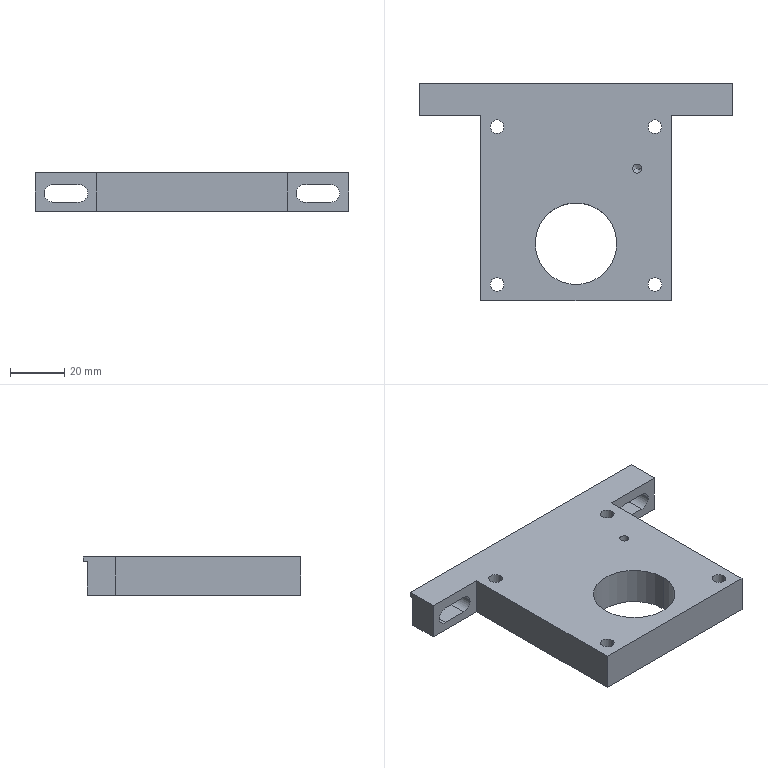Part | NX | features BREP 1 | 1 solid | 36 faces | box 115 x 80 x 14 mm | volume 70777 mm3 | cylinder 18 | plane 16 | cone 2 | commonest cylinder face diameters 5 x8 6.5 x6 3.3 x2 30 x2
STEP:
#1=CARTESIAN_POINT('',(20.814,8.596,-3.1));
#2=VERTEX_POINT('',#1);
#3=CARTESIAN_POINT('',(24.114,8.596,-3.1));
#4=VERTEX_POINT('',#3);
#5=CARTESIAN_POINT('',(22.464,8.596,-3.1));
#6=DIRECTION('',(0.,0.,1.));
#7=DIRECTION('',(1.,0.,0.));
#8=AXIS2_PLACEMENT_3D('',#5,#6,#7);
#9=CIRCLE('',#8,1.65);
#10=EDGE_CURVE('',#2,#4,#9,.T.);
#11=ORIENTED_EDGE('',*,*,#10,.F.);
#12=CARTESIAN_POINT('',(20.814,8.596,7.));
#13=VERTEX_POINT('',#12);
#14=CARTESIAN_POINT('',(20.814,8.596,7.));
#15=DIRECTION('',(0.,0.,1.));
#16=VECTOR('',#15,1000.);
#17=LINE('',#14,#16);
#18=EDGE_CURVE('',#13,#2,#17,.F.);
#19=ORIENTED_EDGE('',*,*,#18,.F.);
#20=CARTESIAN_POINT('',(24.114,8.596,7.));
#21=VERTEX_POINT('',#20);
#22=CARTESIAN_POINT('',(22.464,8.596,7.));
#23=DIRECTION('',(0.,0.,1.));
#24=DIRECTION('',(1.,0.,0.));
#25=AXIS2_PLACEMENT_3D('',#22,#23,#24);
#26=CIRCLE('',#25,1.65);
#27=EDGE_CURVE('',#13,#21,#26,.T.);
#28=ORIENTED_EDGE('',*,*,#27,.T.);
#29=CARTESIAN_POINT('',(24.114,8.596,7.));
#30=DIRECTION('',(0.,0.,1.));
#31=VECTOR('',#30,1000.);
#32=LINE('',#29,#31);
#33=EDGE_CURVE('',#21,#4,#32,.F.);
#34=ORIENTED_EDGE('',*,*,#33,.T.);
#35=EDGE_LOOP('',(#11,#19,#28,#34));
#36=FACE_BOUND('',#35,.T.);
#37=CARTESIAN_POINT('',(22.464,8.596,7.));
#38=DIRECTION('',(0.,0.,1.));
#39=DIRECTION('',(1.,0.,0.));
#40=AXIS2_PLACEMENT_3D('',#37,#38,#39);
#41=CYLINDRICAL_SURFACE('',#40,1.65);
#42=ADVANCED_FACE('',(#36),#41,.F.);
#43=CARTESIAN_POINT('',(22.464,8.596,-4.091));
#44=VERTEX_POINT('',#43);
#45=CARTESIAN_POINT('',(24.114,8.596,-3.1));
#46=DIRECTION('',(0.8572,0.,0.515));
#47=VECTOR('',#46,1000.);
#48=LINE('',#45,#47);
#49=EDGE_CURVE('',#4,#44,#48,.F.);
#50=ORIENTED_EDGE('',*,*,#49,.T.);
#51=CARTESIAN_POINT('',(20.814,8.596,-3.1));
#52=DIRECTION('',(-0.8572,0.,0.515));
#53=VECTOR('',#52,1000.);
#54=LINE('',#51,#53);
#55=EDGE_CURVE('',#2,#44,#54,.F.);
#56=ORIENTED_EDGE('',*,*,#55,.F.);
#57=ORIENTED_EDGE('',*,*,#10,.T.);
#58=EDGE_LOOP('',(#50,#56,#57));
#59=FACE_BOUND('',#58,.T.);
#60=CARTESIAN_POINT('',(22.464,8.596,-3.1));
#61=DIRECTION('',(0.,0.,1.));
#62=DIRECTION('',(1.,0.,0.));
#63=AXIS2_PLACEMENT_3D('',#60,#61,#62);
#64=CONICAL_SURFACE('',#63,1.65,1.03);
#65=ADVANCED_FACE('',(#59),#64,.F.);
#66=CARTESIAN_POINT('',(-38.25,38.5,-0.5));
#67=VERTEX_POINT('',#66);
#68=CARTESIAN_POINT('',(-41.5,38.5,2.75));
#69=VERTEX_POINT('',#68);
#70=CARTESIAN_POINT('',(-41.5,38.5,-0.5));
#71=DIRECTION('',(0.,-1.,0.));
#72=DIRECTION('',(0.,0.,-1.));
#73=AXIS2_PLACEMENT_3D('',#70,#71,#72);
#74=CIRCLE('',#73,3.25);
#75=EDGE_CURVE('',#67,#69,#74,.T.);
#76=ORIENTED_EDGE('',*,*,#75,.F.);
#77=CARTESIAN_POINT('',(-38.25,28.,-0.5));
#78=VERTEX_POINT('',#77);
#79=CARTESIAN_POINT('',(-38.25,40.,-0.5));
#80=DIRECTION('',(0.,-1.,0.));
#81=VECTOR('',#80,1000.);
#82=LINE('',#79,#81);
#83=EDGE_CURVE('',#67,#78,#82,.T.);
#84=ORIENTED_EDGE('',*,*,#83,.T.);
#85=CARTESIAN_POINT('',(-41.5,28.,2.75));
#86=VERTEX_POINT('',#85);
#87=CARTESIAN_POINT('',(-41.5,28.,-0.5));
#88=DIRECTION('',(0.,-1.,0.));
#89=DIRECTION('',(-1.,0.,0.));
#90=AXIS2_PLACEMENT_3D('',#87,#88,#89);
#91=CIRCLE('',#90,3.25);
#92=EDGE_CURVE('',#78,#86,#91,.T.);
#93=ORIENTED_EDGE('',*,*,#92,.T.);
#94=CARTESIAN_POINT('',(-41.5,40.,2.75));
#95=DIRECTION('',(0.,-1.,0.));
#96=VECTOR('',#95,1000.);
#97=LINE('',#94,#96);
#98=EDGE_CURVE('',#69,#86,#97,.T.);
#99=ORIENTED_EDGE('',*,*,#98,.F.);
#100=EDGE_LOOP('',(#76,#84,#93,#99));
#101=FACE_BOUND('',#100,.T.);
#102=CARTESIAN_POINT('',(-41.5,40.,-0.5));
#103=DIRECTION('',(0.,-1.,0.));
#104=DIRECTION('',(1.,0.,0.));
#105=AXIS2_PLACEMENT_3D('',#102,#103,#104);
#106=CYLINDRICAL_SURFACE('',#105,3.25);
#107=ADVANCED_FACE('',(#101),#106,.F.);
#108=CARTESIAN_POINT('',(54.25,38.5,-0.5));
#109=VERTEX_POINT('',#108);
#110=CARTESIAN_POINT('',(51.,38.5,2.75));
#111=VERTEX_POINT('',#110);
#112=CARTESIAN_POINT('',(51.,38.5,-0.5));
#113=DIRECTION('',(0.,-1.,0.));
#114=DIRECTION('',(0.,0.,-1.));
#115=AXIS2_PLACEMENT_3D('',#112,#113,#114);
#116=CIRCLE('',#115,3.25);
#117=EDGE_CURVE('',#109,#111,#116,.T.);
#118=ORIENTED_EDGE('',*,*,#117,.F.);
#119=CARTESIAN_POINT('',(54.25,28.,-0.5));
#120=VERTEX_POINT('',#119);
#121=CARTESIAN_POINT('',(54.25,40.,-0.5));
#122=DIRECTION('',(0.,-1.,0.));
#123=VECTOR('',#122,1000.);
#124=LINE('',#121,#123);
#125=EDGE_CURVE('',#109,#120,#124,.T.);
#126=ORIENTED_EDGE('',*,*,#125,.T.);
#127=CARTESIAN_POINT('',(51.,28.,2.75));
#128=VERTEX_POINT('',#127);
#129=CARTESIAN_POINT('',(51.,28.,-0.5));
#130=DIRECTION('',(0.,-1.,0.));
#131=DIRECTION('',(1.,0.,0.));
#132=AXIS2_PLACEMENT_3D('',#129,#130,#131);
#133=CIRCLE('',#132,3.25);
#134=EDGE_CURVE('',#120,#128,#133,.T.);
#135=ORIENTED_EDGE('',*,*,#134,.T.);
#136=CARTESIAN_POINT('',(51.,40.,2.75));
#137=DIRECTION('',(0.,-1.,0.));
#138=VECTOR('',#137,1000.);
#139=LINE('',#136,#138);
#140=EDGE_CURVE('',#111,#128,#139,.T.);
#141=ORIENTED_EDGE('',*,*,#140,.F.);
#142=EDGE_LOOP('',(#118,#126,#135,#141));
#143=FACE_BOUND('',#142,.T.);
#144=CARTESIAN_POINT('',(51.,40.,-0.5));
#145=DIRECTION('',(0.,-1.,0.));
#146=DIRECTION('',(1.,0.,0.));
#147=AXIS2_PLACEMENT_3D('',#144,#145,#146);
#148=CYLINDRICAL_SURFACE('',#147,3.25);
#149=ADVANCED_FACE('',(#143),#148,.F.);
#150=CARTESIAN_POINT('',(26.491,23.991,-7.));
#151=VERTEX_POINT('',#150);
#152=CARTESIAN_POINT('',(31.491,23.991,-7.));
#153=VERTEX_POINT('',#152);
#154=CARTESIAN_POINT('',(28.991,23.991,-7.));
#155=DIRECTION('',(0.,0.,1.));
#156=DIRECTION('',(1.,0.,0.));
#157=AXIS2_PLACEMENT_3D('',#154,#155,#156);
#158=CIRCLE('',#157,2.5);
#159=EDGE_CURVE('',#151,#153,#158,.T.);
#160=ORIENTED_EDGE('',*,*,#159,.F.);
#161=CARTESIAN_POINT('',(26.491,23.991,7.));
#162=VERTEX_POINT('',#161);
#163=CARTESIAN_POINT('',(26.491,23.991,7.));
#164=DIRECTION('',(0.,0.,1.));
#165=VECTOR('',#164,1000.);
#166=LINE('',#163,#165);
#167=EDGE_CURVE('',#162,#151,#166,.F.);
#168=ORIENTED_EDGE('',*,*,#167,.F.);
#169=CARTESIAN_POINT('',(31.491,23.991,7.));
#170=VERTEX_POINT('',#169);
#171=CARTESIAN_POINT('',(28.991,23.991,7.));
#172=DIRECTION('',(0.,0.,1.));
#173=DIRECTION('',(1.,0.,0.));
#174=AXIS2_PLACEMENT_3D('',#171,#172,#173);
#175=CIRCLE('',#174,2.5);
#176=EDGE_CURVE('',#162,#170,#175,.T.);
#177=ORIENTED_EDGE('',*,*,#176,.T.);
#178=CARTESIAN_POINT('',(31.491,23.991,7.));
#179=DIRECTION('',(0.,0.,1.));
#180=VECTOR('',#179,1000.);
#181=LINE('',#178,#180);
#182=EDGE_CURVE('',#170,#153,#181,.F.);
#183=ORIENTED_EDGE('',*,*,#182,.T.);
#184=EDGE_LOOP('',(#160,#168,#177,#183));
#185=FACE_BOUND('',#184,.T.);
#186=CARTESIAN_POINT('',(28.991,23.991,7.));
#187=DIRECTION('',(0.,0.,1.));
#188=DIRECTION('',(1.,0.,0.));
#189=AXIS2_PLACEMENT_3D('',#186,#187,#188);
#190=CYLINDRICAL_SURFACE('',#189,2.5);
#191=ADVANCED_FACE('',(#185),#190,.F.);
#192=CARTESIAN_POINT('',(-31.491,23.991,-7.));
#193=VERTEX_POINT('',#192);
#194=CARTESIAN_POINT('',(-26.491,23.991,-7.));
#195=VERTEX_POINT('',#194);
#196=CARTESIAN_POINT('',(-28.991,23.991,-7.));
#197=DIRECTION('',(0.,0.,1.));
#198=DIRECTION('',(1.,0.,0.));
#199=AXIS2_PLACEMENT_3D('',#196,#197,#198);
#200=CIRCLE('',#199,2.5);
#201=EDGE_CURVE('',#193,#195,#200,.T.);
#202=ORIENTED_EDGE('',*,*,#201,.F.);
#203=CARTESIAN_POINT('',(-31.491,23.991,7.));
#204=VERTEX_POINT('',#203);
#205=CARTESIAN_POINT('',(-31.491,23.991,7.));
#206=DIRECTION('',(0.,0.,1.));
#207=VECTOR('',#206,1000.);
#208=LINE('',#205,#207);
#209=EDGE_CURVE('',#204,#193,#208,.F.);
#210=ORIENTED_EDGE('',*,*,#209,.F.);
#211=CARTESIAN_POINT('',(-26.491,23.991,7.));
#212=VERTEX_POINT('',#211);
#213=CARTESIAN_POINT('',(-28.991,23.991,7.));
#214=DIRECTION('',(0.,0.,1.));
#215=DIRECTION('',(1.,0.,0.));
#216=AXIS2_PLACEMENT_3D('',#213,#214,#215);
#217=CIRCLE('',#216,2.5);
#218=EDGE_CURVE('',#204,#212,#217,.T.);
#219=ORIENTED_EDGE('',*,*,#218,.T.);
#220=CARTESIAN_POINT('',(-26.491,23.991,7.));
#221=DIRECTION('',(0.,0.,1.));
#222=VECTOR('',#221,1000.);
#223=LINE('',#220,#222);
#224=EDGE_CURVE('',#212,#195,#223,.F.);
#225=ORIENTED_EDGE('',*,*,#224,.T.);
#226=EDGE_LOOP('',(#202,#210,#219,#225));
#227=FACE_BOUND('',#226,.T.);
#228=CARTESIAN_POINT('',(-28.991,23.991,7.));
#229=DIRECTION('',(0.,0.,1.));
#230=DIRECTION('',(1.,0.,0.));
#231=AXIS2_PLACEMENT_3D('',#228,#229,#230);
#232=CYLINDRICAL_SURFACE('',#231,2.5);
#233=ADVANCED_FACE('',(#227),#232,.F.);
#234=CARTESIAN_POINT('',(26.491,-33.991,-7.));
#235=VERTEX_POINT('',#234);
#236=CARTESIAN_POINT('',(31.491,-33.991,-7.));
#237=VERTEX_POINT('',#236);
#238=CARTESIAN_POINT('',(28.991,-33.991,-7.));
#239=DIRECTION('',(0.,0.,1.));
#240=DIRECTION('',(1.,0.,0.));
#241=AXIS2_PLACEMENT_3D('',#238,#239,#240);
#242=CIRCLE('',#241,2.5);
#243=EDGE_CURVE('',#235,#237,#242,.T.);
#244=ORIENTED_EDGE('',*,*,#243,.F.);
#245=CARTESIAN_POINT('',(26.491,-33.991,7.));
#246=VERTEX_POINT('',#245);
#247=CARTESIAN_POINT('',(26.491,-33.991,7.));
#248=DIRECTION('',(0.,0.,1.));
#249=VECTOR('',#248,1000.);
#250=LINE('',#247,#249);
#251=EDGE_CURVE('',#246,#235,#250,.F.);
#252=ORIENTED_EDGE('',*,*,#251,.F.);
#253=CARTESIAN_POINT('',(31.491,-33.991,7.));
#254=VERTEX_POINT('',#253);
#255=CARTESIAN_POINT('',(28.991,-33.991,7.));
#256=DIRECTION('',(0.,0.,1.));
#257=DIRECTION('',(1.,0.,0.));
#258=AXIS2_PLACEMENT_3D('',#255,#256,#257);
#259=CIRCLE('',#258,2.5);
#260=EDGE_CURVE('',#246,#254,#259,.T.);
#261=ORIENTED_EDGE('',*,*,#260,.T.);
#262=CARTESIAN_POINT('',(31.491,-33.991,7.));
#263=DIRECTION('',(0.,0.,1.));
#264=VECTOR('',#263,1000.);
#265=LINE('',#262,#264);
#266=EDGE_CURVE('',#254,#237,#265,.F.);
#267=ORIENTED_EDGE('',*,*,#266,.T.);
#268=EDGE_LOOP('',(#244,#252,#261,#267));
#269=FACE_BOUND('',#268,.T.);
#270=CARTESIAN_POINT('',(28.991,-33.991,7.));
#271=DIRECTION('',(0.,0.,1.));
#272=DIRECTION('',(1.,0.,0.));
#273=AXIS2_PLACEMENT_3D('',#270,#271,#272);
#274=CYLINDRICAL_SURFACE('',#273,2.5);
#275=ADVANCED_FACE('',(#269),#274,.F.);
#276=CARTESIAN_POINT('',(-31.491,-33.991,-7.));
#277=VERTEX_POINT('',#276);
#278=CARTESIAN_POINT('',(-26.491,-33.991,-7.));
#279=VERTEX_POINT('',#278);
#280=CARTESIAN_POINT('',(-28.991,-33.991,-7.));
#281=DIRECTION('',(0.,0.,1.));
#282=DIRECTION('',(1.,0.,0.));
#283=AXIS2_PLACEMENT_3D('',#280,#281,#282);
#284=CIRCLE('',#283,2.5);
#285=EDGE_CURVE('',#277,#279,#284,.T.);
#286=ORIENTED_EDGE('',*,*,#285,.F.);
#287=CARTESIAN_POINT('',(-31.491,-33.991,7.));
#288=VERTEX_POINT('',#287);
#289=CARTESIAN_POINT('',(-31.491,-33.991,7.));
#290=DIRECTION('',(0.,0.,1.));
#291=VECTOR('',#290,1000.);
#292=LINE('',#289,#291);
#293=EDGE_CURVE('',#288,#277,#292,.F.);
#294=ORIENTED_EDGE('',*,*,#293,.F.);
#295=CARTESIAN_POINT('',(-26.491,-33.991,7.));
#296=VERTEX_POINT('',#295);
#297=CARTESIAN_POINT('',(-28.991,-33.991,7.));
#298=DIRECTION('',(0.,0.,1.));
#299=DIRECTION('',(1.,0.,0.));
#300=AXIS2_PLACEMENT_3D('',#297,#298,#299);
#301=CIRCLE('',#300,2.5);
#302=EDGE_CURVE('',#288,#296,#301,.T.);
#303=ORIENTED_EDGE('',*,*,#302,.T.);
#304=CARTESIAN_POINT('',(-26.491,-33.991,7.));
#305=DIRECTION('',(0.,0.,1.));
#306=VECTOR('',#305,1000.);
#307=LINE('',#304,#306);
#308=EDGE_CURVE('',#296,#279,#307,.F.);
#309=ORIENTED_EDGE('',*,*,#308,.T.);
#310=EDGE_LOOP('',(#286,#294,#303,#309));
#311=FACE_BOUND('',#310,.T.);
#312=CARTESIAN_POINT('',(-28.991,-33.991,7.));
#313=DIRECTION('',(0.,0.,1.));
#314=DIRECTION('',(1.,0.,0.));
#315=AXIS2_PLACEMENT_3D('',#312,#313,#314);
#316=CYLINDRICAL_SURFACE('',#315,2.5);
#317=ADVANCED_FACE('',(#311),#316,.F.);
#318=CARTESIAN_POINT('',(15.,-19.,7.));
#319=VERTEX_POINT('',#318);
#320=CARTESIAN_POINT('',(-15.,-19.,7.));
#321=VERTEX_POINT('',#320);
#322=CARTESIAN_POINT('',(0.,-19.,7.));
#323=DIRECTION('',(0.,0.,-1.));
#324=DIRECTION('',(-1.,0.,0.));
#325=AXIS2_PLACEMENT_3D('',#322,#323,#324);
#326=CIRCLE('',#325,15.);
#327=EDGE_CURVE('',#319,#321,#326,.T.);
#328=ORIENTED_EDGE('',*,*,#327,.F.);
#329=CARTESIAN_POINT('',(15.,-19.,-7.));
#330=VERTEX_POINT('',#329);
#331=CARTESIAN_POINT('',(15.,-19.,7.));
#332=DIRECTION('',(0.,0.,-1.));
#333=VECTOR('',#332,1000.);
#334=LINE('',#331,#333);
#335=EDGE_CURVE('',#319,#330,#334,.T.);
#336=ORIENTED_EDGE('',*,*,#335,.T.);
#337=CARTESIAN_POINT('',(-15.,-19.,-7.));
#338=VERTEX_POINT('',#337);
#339=CARTESIAN_POINT('',(0.,-19.,-7.));
#340=DIRECTION('',(0.,0.,-1.));
#341=DIRECTION('',(-1.,0.,0.));
#342=AXIS2_PLACEMENT_3D('',#339,#340,#341);
#343=CIRCLE('',#342,15.);
#344=EDGE_CURVE('',#330,#338,#343,.T.);
#345=ORIENTED_EDGE('',*,*,#344,.T.);
#346=CARTESIAN_POINT('',(-15.,-19.,7.));
#347=DIRECTION('',(0.,0.,-1.));
#348=VECTOR('',#347,1000.);
#349=LINE('',#346,#348);
#350=EDGE_CURVE('',#321,#338,#349,.T.);
#351=ORIENTED_EDGE('',*,*,#350,.F.);
#352=EDGE_LOOP('',(#328,#336,#345,#351));
#353=FACE_BOUND('',#352,.T.);
#354=CARTESIAN_POINT('',(0.,-19.,7.));
#355=DIRECTION('',(0.,0.,-1.));
#356=DIRECTION('',(-1.,0.,0.));
#357=AXIS2_PLACEMENT_3D('',#354,#355,#356);
#358=CYLINDRICAL_SURFACE('',#357,15.);
#359=ADVANCED_FACE('',(#353),#358,.F.);
#360=CARTESIAN_POINT('',(-57.5,38.5,-7.));
#361=VERTEX_POINT('',#360);
#362=CARTESIAN_POINT('',(-57.5,28.,-7.));
#363=VERTEX_POINT('',#362);
#364=CARTESIAN_POINT('',(-57.5,40.,-7.));
#365=DIRECTION('',(0.,-1.,0.));
#366=VECTOR('',#365,1000.);
#367=LINE('',#364,#366);
#368=EDGE_CURVE('',#361,#363,#367,.T.);
#369=ORIENTED_EDGE('',*,*,#368,.T.);
#370=CARTESIAN_POINT('',(-57.5,28.,7.));
#371=VERTEX_POINT('',#370);
#372=CARTESIAN_POINT('',(-57.5,28.,-7.));
#373=DIRECTION('',(0.,0.,1.));
#374=VECTOR('',#373,1000.);
#375=LINE('',#372,#374);
#376=EDGE_CURVE('',#363,#371,#375,.T.);
#377=ORIENTED_EDGE('',*,*,#376,.T.);
#378=CARTESIAN_POINT('',(-57.5,40.,7.));
#379=VERTEX_POINT('',#378);
#380=CARTESIAN_POINT('',(-57.5,40.,7.));
#381=DIRECTION('',(0.,-1.,0.));
#382=VECTOR('',#381,1000.);
#383=LINE('',#380,#382);
#384=EDGE_CURVE('',#379,#371,#383,.T.);
#385=ORIENTED_EDGE('',*,*,#384,.F.);
#386=CARTESIAN_POINT('',(-57.5,40.,5.2));
#387=VERTEX_POINT('',#386);
#388=CARTESIAN_POINT('',(-57.5,40.,-7.));
#389=DIRECTION('',(0.,0.,1.));
#390=VECTOR('',#389,1000.);
#391=LINE('',#388,#390);
#392=EDGE_CURVE('',#387,#379,#391,.T.);
#393=ORIENTED_EDGE('',*,*,#392,.F.);
#394=CARTESIAN_POINT('',(-57.5,38.5,5.2));
#395=VERTEX_POINT('',#394);
#396=CARTESIAN_POINT('',(-57.5,40.,5.2));
#397=DIRECTION('',(0.,-1.,0.));
#398=VECTOR('',#397,1000.);
#399=LINE('',#396,#398);
#400=EDGE_CURVE('',#387,#395,#399,.T.);
#401=ORIENTED_EDGE('',*,*,#400,.T.);
#402=CARTESIAN_POINT('',(-57.5,38.5,-7.));
#403=DIRECTION('',(0.,0.,-1.));
#404=VECTOR('',#403,1000.);
#405=LINE('',#402,#404);
#406=EDGE_CURVE('',#395,#361,#405,.T.);
#407=ORIENTED_EDGE('',*,*,#406,.T.);
#408=EDGE_LOOP('',(#369,#377,#385,#393,#401,#407));
#409=FACE_BOUND('',#408,.T.);
#410=CARTESIAN_POINT('',(-57.5,40.,-7.));
#411=DIRECTION('',(1.,0.,0.));
#412=DIRECTION('',(0.,1.,0.));
#413=AXIS2_PLACEMENT_3D('',#410,#411,#412);
#414=PLANE('',#413);
#415=ADVANCED_FACE('',(#409),#414,.F.);
#416=CARTESIAN_POINT('',(-35.,-40.,7.));
#417=VERTEX_POINT('',#416);
#418=CARTESIAN_POINT('',(35.,-40.,7.));
#419=VERTEX_POINT('',#418);
#420=CARTESIAN_POINT('',(-57.5,-40.,7.));
#421=DIRECTION('',(1.,0.,0.));
#422=VECTOR('',#421,1000.);
#423=LINE('',#420,#422);
#424=EDGE_CURVE('',#417,#419,#423,.T.);
#425=ORIENTED_EDGE('',*,*,#424,.T.);
#426=CARTESIAN_POINT('',(35.,28.,7.));
#427=VERTEX_POINT('',#426);
#428=CARTESIAN_POINT('',(35.,-40.,7.));
#429=DIRECTION('',(0.,-1.,0.));
#430=VECTOR('',#429,1000.);
#431=LINE('',#428,#430);
#432=EDGE_CURVE('',#427,#419,#431,.T.);
#433=ORIENTED_EDGE('',*,*,#432,.F.);
#434=CARTESIAN_POINT('',(57.5,28.,7.));
#435=VERTEX_POINT('',#434);
#436=CARTESIAN_POINT('',(57.5,28.,7.));
#437=DIRECTION('',(-1.,0.,0.));
#438=VECTOR('',#437,1000.);
#439=LINE('',#436,#438);
#440=EDGE_CURVE('',#435,#427,#439,.T.);
#441=ORIENTED_EDGE('',*,*,#440,.F.);
#442=CARTESIAN_POINT('',(57.5,40.,7.));
#443=VERTEX_POINT('',#442);
#444=CARTESIAN_POINT('',(57.5,40.,7.));
#445=DIRECTION('',(0.,-1.,0.));
#446=VECTOR('',#445,1000.);
#447=LINE('',#444,#446);
#448=EDGE_CURVE('',#443,#435,#447,.T.);
#449=ORIENTED_EDGE('',*,*,#448,.F.);
#450=CARTESIAN_POINT('',(-57.5,40.,7.));
#451=DIRECTION('',(1.,0.,0.));
#452=VECTOR('',#451,1000.);
#453=LINE('',#450,#452);
#454=EDGE_CURVE('',#379,#443,#453,.T.);
#455=ORIENTED_EDGE('',*,*,#454,.F.);
#456=ORIENTED_EDGE('',*,*,#384,.T.);
#457=CARTESIAN_POINT('',(-35.,28.,7.));
#458=VERTEX_POINT('',#457);
#459=CARTESIAN_POINT('',(-57.5,28.,7.));
#460=DIRECTION('',(-1.,0.,0.));
#461=VECTOR('',#460,1000.);
#462=LINE('',#459,#461);
#463=EDGE_CURVE('',#458,#371,#462,.T.);
#464=ORIENTED_EDGE('',*,*,#463,.F.);
#465=CARTESIAN_POINT('',(-35.,-40.,7.));
#466=DIRECTION('',(0.,1.,0.));
#467=VECTOR('',#466,1000.);
#468=LINE('',#465,#467);
#469=EDGE_CURVE('',#417,#458,#468,.T.);
#470=ORIENTED_EDGE('',*,*,#469,.F.);
#471=EDGE_LOOP('',(#425,#433,#441,#449,#455,#456,#464,#470));
#472=FACE_BOUND('',#471,.T.);
#473=CARTESIAN_POINT('',(22.464,8.596,7.));
#474=DIRECTION('',(0.,0.,1.));
#475=DIRECTION('',(1.,0.,0.));
#476=AXIS2_PLACEMENT_3D('',#473,#474,#475);
#477=CIRCLE('',#476,1.65);
#478=EDGE_CURVE('',#21,#13,#477,.T.);
#479=ORIENTED_EDGE('',*,*,#478,.F.);
#480=ORIENTED_EDGE('',*,*,#27,.F.);
#481=EDGE_LOOP('',(#479,#480));
#482=FACE_BOUND('',#481,.T.);
#483=CARTESIAN_POINT('',(28.991,23.991,7.));
#484=DIRECTION('',(0.,0.,1.));
#485=DIRECTION('',(1.,0.,0.));
#486=AXIS2_PLACEMENT_3D('',#483,#484,#485);
#487=CIRCLE('',#486,2.5);
#488=EDGE_CURVE('',#170,#162,#487,.T.);
#489=ORIENTED_EDGE('',*,*,#488,.F.);
#490=ORIENTED_EDGE('',*,*,#176,.F.);
#491=EDGE_LOOP('',(#489,#490));
#492=FACE_BOUND('',#491,.T.);
#493=CARTESIAN_POINT('',(-28.991,23.991,7.));
#494=DIRECTION('',(0.,0.,1.));
#495=DIRECTION('',(1.,0.,0.));
#496=AXIS2_PLACEMENT_3D('',#493,#494,#495);
#497=CIRCLE('',#496,2.5);
#498=EDGE_CURVE('',#212,#204,#497,.T.);
#499=ORIENTED_EDGE('',*,*,#498,.F.);
#500=ORIENTED_EDGE('',*,*,#218,.F.);
#501=EDGE_LOOP('',(#499,#500));
#502=FACE_BOUND('',#501,.T.);
#503=CARTESIAN_POINT('',(28.991,-33.991,7.));
#504=DIRECTION('',(0.,0.,1.));
#505=DIRECTION('',(1.,0.,0.));
#506=AXIS2_PLACEMENT_3D('',#503,#504,#505);
#507=CIRCLE('',#506,2.5);
#508=EDGE_CURVE('',#254,#246,#507,.T.);
#509=ORIENTED_EDGE('',*,*,#508,.F.);
#510=ORIENTED_EDGE('',*,*,#260,.F.);
#511=EDGE_LOOP('',(#509,#510));
#512=FACE_BOUND('',#511,.T.);
#513=CARTESIAN_POINT('',(-28.991,-33.991,7.));
#514=DIRECTION('',(0.,0.,1.));
#515=DIRECTION('',(1.,0.,0.));
#516=AXIS2_PLACEMENT_3D('',#513,#514,#515);
#517=CIRCLE('',#516,2.5);
#518=EDGE_CURVE('',#296,#288,#517,.T.);
#519=ORIENTED_EDGE('',*,*,#518,.F.);
#520=ORIENTED_EDGE('',*,*,#302,.F.);
#521=EDGE_LOOP('',(#519,#520));
#522=FACE_BOUND('',#521,.T.);
#523=CARTESIAN_POINT('',(0.,-19.,7.));
#524=DIRECTION('',(0.,0.,-1.));
#525=DIRECTION('',(-1.,0.,0.));
#526=AXIS2_PLACEMENT_3D('',#523,#524,#525);
#527=CIRCLE('',#526,15.);
#528=EDGE_CURVE('',#321,#319,#527,.T.);
#529=ORIENTED_EDGE('',*,*,#528,.T.);
#530=ORIENTED_EDGE('',*,*,#327,.T.);
#531=EDGE_LOOP('',(#529,#530));
#532=FACE_BOUND('',#531,.T.);
#533=CARTESIAN_POINT('',(-57.5,40.,7.));
#534=DIRECTION('',(0.,0.,-1.));
#535=DIRECTION('',(0.,-1.,0.));
#536=AXIS2_PLACEMENT_3D('',#533,#534,#535);
#537=PLANE('',#536);
#538=ADVANCED_FACE('',(#472,#482,#492,#502,#512,#522,#532),#537,.F.);
#539=ORIENTED_EDGE('',*,*,#448,.T.);
#540=CARTESIAN_POINT('',(57.5,28.,-7.));
#541=VERTEX_POINT('',#540);
#542=CARTESIAN_POINT('',(57.5,28.,-7.));
#543=DIRECTION('',(0.,0.,1.));
#544=VECTOR('',#543,1000.);
#545=LINE('',#542,#544);
#546=EDGE_CURVE('',#541,#435,#545,.T.);
#547=ORIENTED_EDGE('',*,*,#546,.F.);
#548=CARTESIAN_POINT('',(57.5,38.5,-7.));
#549=VERTEX_POINT('',#548);
#550=CARTESIAN_POINT('',(57.5,40.,-7.));
#551=DIRECTION('',(0.,-1.,0.));
#552=VECTOR('',#551,1000.);
#553=LINE('',#550,#552);
#554=EDGE_CURVE('',#549,#541,#553,.T.);
#555=ORIENTED_EDGE('',*,*,#554,.F.);
#556=CARTESIAN_POINT('',(57.5,38.5,5.2));
#557=VERTEX_POINT('',#556);
#558=CARTESIAN_POINT('',(57.5,38.5,-7.));
#559=DIRECTION('',(0.,0.,-1.));
#560=VECTOR('',#559,1000.);
#561=LINE('',#558,#560);
#562=EDGE_CURVE('',#557,#549,#561,.T.);
#563=ORIENTED_EDGE('',*,*,#562,.F.);
#564=CARTESIAN_POINT('',(57.5,40.,5.2));
#565=VERTEX_POINT('',#564);
#566=CARTESIAN_POINT('',(57.5,40.,5.2));
#567=DIRECTION('',(0.,-1.,0.));
#568=VECTOR('',#567,1000.);
#569=LINE('',#566,#568);
#570=EDGE_CURVE('',#565,#557,#569,.T.);
#571=ORIENTED_EDGE('',*,*,#570,.F.);
#572=CARTESIAN_POINT('',(57.5,40.,-7.));
#573=DIRECTION('',(0.,0.,-1.));
#574=VECTOR('',#573,1000.);
#575=LINE('',#572,#574);
#576=EDGE_CURVE('',#443,#565,#575,.T.);
#577=ORIENTED_EDGE('',*,*,#576,.F.);
#578=EDGE_LOOP('',(#539,#547,#555,#563,#571,#577));
#579=FACE_BOUND('',#578,.T.);
#580=CARTESIAN_POINT('',(57.5,40.,-7.));
#581=DIRECTION('',(-1.,0.,0.));
#582=DIRECTION('',(0.,0.,1.));
#583=AXIS2_PLACEMENT_3D('',#580,#581,#582);
#584=PLANE('',#583);
#585=ADVANCED_FACE('',(#579),#584,.F.);
#586=CARTESIAN_POINT('',(35.,28.,-7.));
#587=VERTEX_POINT('',#586);
#588=CARTESIAN_POINT('',(57.5,28.,-7.));
#589=DIRECTION('',(-1.,0.,0.));
#590=VECTOR('',#589,1000.);
#591=LINE('',#588,#590);
#592=EDGE_CURVE('',#541,#587,#591,.T.);
#593=ORIENTED_EDGE('',*,*,#592,.T.);
#594=CARTESIAN_POINT('',(35.,-40.,-7.));
#595=VERTEX_POINT('',#594);
#596=CARTESIAN_POINT('',(35.,-40.,-7.));
#597=DIRECTION('',(0.,-1.,0.));
#598=VECTOR('',#597,1000.);
#599=LINE('',#596,#598);
#600=EDGE_CURVE('',#587,#595,#599,.T.);
#601=ORIENTED_EDGE('',*,*,#600,.T.);
#602=CARTESIAN_POINT('',(-35.,-40.,-7.));
#603=VERTEX_POINT('',#602);
#604=CARTESIAN_POINT('',(-57.5,-40.,-7.));
#605=DIRECTION('',(-1.,0.,0.));
#606=VECTOR('',#605,1000.);
#607=LINE('',#604,#606);
#608=EDGE_CURVE('',#595,#603,#607,.T.);
#609=ORIENTED_EDGE('',*,*,#608,.T.);
#610=CARTESIAN_POINT('',(-35.,28.,-7.));
#611=VERTEX_POINT('',#610);
#612=CARTESIAN_POINT('',(-35.,-40.,-7.));
#613=DIRECTION('',(0.,1.,0.));
#614=VECTOR('',#613,1000.);
#615=LINE('',#612,#614);
#616=EDGE_CURVE('',#603,#611,#615,.T.);
#617=ORIENTED_EDGE('',*,*,#616,.T.);
#618=CARTESIAN_POINT('',(-57.5,28.,-7.));
#619=DIRECTION('',(-1.,0.,0.));
#620=VECTOR('',#619,1000.);
#621=LINE('',#618,#620);
#622=EDGE_CURVE('',#611,#363,#621,.T.);
#623=ORIENTED_EDGE('',*,*,#622,.T.);
#624=ORIENTED_EDGE('',*,*,#368,.F.);
#625=CARTESIAN_POINT('',(-57.5,38.5,-7.));
#626=DIRECTION('',(1.,0.,0.));
#627=VECTOR('',#626,1000.);
#628=LINE('',#625,#627);
#629=EDGE_CURVE('',#361,#549,#628,.T.);
#630=ORIENTED_EDGE('',*,*,#629,.T.);
#631=ORIENTED_EDGE('',*,*,#554,.T.);
#632=EDGE_LOOP('',(#593,#601,#609,#617,#623,#624,#630,#631));
#633=FACE_BOUND('',#632,.T.);
#634=CARTESIAN_POINT('',(28.991,23.991,-7.));
#635=DIRECTION('',(0.,0.,1.));
#636=DIRECTION('',(1.,0.,0.));
#637=AXIS2_PLACEMENT_3D('',#634,#635,#636);
#638=CIRCLE('',#637,2.5);
#639=EDGE_CURVE('',#153,#151,#638,.T.);
#640=ORIENTED_EDGE('',*,*,#639,.T.);
#641=ORIENTED_EDGE('',*,*,#159,.T.);
#642=EDGE_LOOP('',(#640,#641));
#643=FACE_BOUND('',#642,.T.);
#644=CARTESIAN_POINT('',(-28.991,23.991,-7.));
#645=DIRECTION('',(0.,0.,1.));
#646=DIRECTION('',(1.,0.,0.));
#647=AXIS2_PLACEMENT_3D('',#644,#645,#646);
#648=CIRCLE('',#647,2.5);
#649=EDGE_CURVE('',#195,#193,#648,.T.);
#650=ORIENTED_EDGE('',*,*,#649,.T.);
#651=ORIENTED_EDGE('',*,*,#201,.T.);
#652=EDGE_LOOP('',(#650,#651));
#653=FACE_BOUND('',#652,.T.);
#654=CARTESIAN_POINT('',(28.991,-33.991,-7.));
#655=DIRECTION('',(0.,0.,1.));
#656=DIRECTION('',(1.,0.,0.));
#657=AXIS2_PLACEMENT_3D('',#654,#655,#656);
#658=CIRCLE('',#657,2.5);
#659=EDGE_CURVE('',#237,#235,#658,.T.);
#660=ORIENTED_EDGE('',*,*,#659,.T.);
#661=ORIENTED_EDGE('',*,*,#243,.T.);
#662=EDGE_LOOP('',(#660,#661));
#663=FACE_BOUND('',#662,.T.);
#664=CARTESIAN_POINT('',(-28.991,-33.991,-7.));
#665=DIRECTION('',(0.,0.,1.));
#666=DIRECTION('',(1.,0.,0.));
#667=AXIS2_PLACEMENT_3D('',#664,#665,#666);
#668=CIRCLE('',#667,2.5);
#669=EDGE_CURVE('',#279,#277,#668,.T.);
#670=ORIENTED_EDGE('',*,*,#669,.T.);
#671=ORIENTED_EDGE('',*,*,#285,.T.);
#672=EDGE_LOOP('',(#670,#671));
#673=FACE_BOUND('',#672,.T.);
#674=CARTESIAN_POINT('',(0.,-19.,-7.));
#675=DIRECTION('',(0.,0.,-1.));
#676=DIRECTION('',(-1.,0.,0.));
#677=AXIS2_PLACEMENT_3D('',#674,#675,#676);
#678=CIRCLE('',#677,15.);
#679=EDGE_CURVE('',#338,#330,#678,.T.);
#680=ORIENTED_EDGE('',*,*,#679,.F.);
#681=ORIENTED_EDGE('',*,*,#344,.F.);
#682=EDGE_LOOP('',(#680,#681));
#683=FACE_BOUND('',#682,.T.);
#684=CARTESIAN_POINT('',(-57.5,40.,-7.));
#685=DIRECTION('',(0.,0.,1.));
#686=DIRECTION('',(1.,0.,0.));
#687=AXIS2_PLACEMENT_3D('',#684,#685,#686);
#688=PLANE('',#687);
#689=ADVANCED_FACE('',(#633,#643,#653,#663,#673,#683),#688,.F.);
#690=CARTESIAN_POINT('',(-57.5,40.,5.2));
#691=DIRECTION('',(1.,0.,0.));
#692=VECTOR('',#691,1000.);
#693=LINE('',#690,#692);
#694=EDGE_CURVE('',#387,#565,#693,.T.);
#695=ORIENTED_EDGE('',*,*,#694,.F.);
#696=ORIENTED_EDGE('',*,*,#392,.T.);
#697=ORIENTED_EDGE('',*,*,#454,.T.);
#698=ORIENTED_EDGE('',*,*,#576,.T.);
#699=EDGE_LOOP('',(#695,#696,#697,#698));
#700=FACE_BOUND('',#699,.T.);
#701=CARTESIAN_POINT('',(-57.5,40.,7.));
#702=DIRECTION('',(0.,1.,0.));
#703=DIRECTION('',(1.,0.,0.));
#704=AXIS2_PLACEMENT_3D('',#701,#702,#703);
#705=PLANE('',#704);
#706=ADVANCED_FACE('',(#700),#705,.T.);
#707=ORIENTED_EDGE('',*,*,#608,.F.);
#708=CARTESIAN_POINT('',(35.,-40.,-7.));
#709=DIRECTION('',(0.,0.,1.));
#710=VECTOR('',#709,1000.);
#711=LINE('',#708,#710);
#712=EDGE_CURVE('',#595,#419,#711,.T.);
#713=ORIENTED_EDGE('',*,*,#712,.T.);
#714=ORIENTED_EDGE('',*,*,#424,.F.);
#715=CARTESIAN_POINT('',(-35.,-40.,-7.));
#716=DIRECTION('',(0.,0.,1.));
#717=VECTOR('',#716,1000.);
#718=LINE('',#715,#717);
#719=EDGE_CURVE('',#603,#417,#718,.T.);
#720=ORIENTED_EDGE('',*,*,#719,.F.);
#721=EDGE_LOOP('',(#707,#713,#714,#720));
#722=FACE_BOUND('',#721,.T.);
#723=CARTESIAN_POINT('',(-57.5,-40.,7.));
#724=DIRECTION('',(0.,1.,0.));
#725=DIRECTION('',(1.,0.,0.));
#726=AXIS2_PLACEMENT_3D('',#723,#724,#725);
#727=PLANE('',#726);
#728=ADVANCED_FACE('',(#722),#727,.F.);
#729=ORIENTED_EDGE('',*,*,#562,.T.);
#730=ORIENTED_EDGE('',*,*,#629,.F.);
#731=ORIENTED_EDGE('',*,*,#406,.F.);
#732=CARTESIAN_POINT('',(-57.5,38.5,5.2));
#733=DIRECTION('',(1.,0.,0.));
#734=VECTOR('',#733,1000.);
#735=LINE('',#732,#734);
#736=EDGE_CURVE('',#395,#557,#735,.T.);
#737=ORIENTED_EDGE('',*,*,#736,.T.);
#738=EDGE_LOOP('',(#729,#730,#731,#737));
#739=FACE_BOUND('',#738,.T.);
#740=CARTESIAN_POINT('',(-51.,38.5,2.75));
#741=VERTEX_POINT('',#740);
#742=CARTESIAN_POINT('',(-57.5,38.5,2.75));
#743=DIRECTION('',(-1.,0.,0.));
#744=VECTOR('',#743,1000.);
#745=LINE('',#742,#744);
#746=EDGE_CURVE('',#69,#741,#745,.T.);
#747=ORIENTED_EDGE('',*,*,#746,.T.);
#748=CARTESIAN_POINT('',(-51.,38.5,-3.75));
#749=VERTEX_POINT('',#748);
#750=CARTESIAN_POINT('',(-51.,38.5,-0.5));
#751=DIRECTION('',(0.,-1.,0.));
#752=DIRECTION('',(0.,0.,-1.));
#753=AXIS2_PLACEMENT_3D('',#750,#751,#752);
#754=CIRCLE('',#753,3.25);
#755=EDGE_CURVE('',#741,#749,#754,.T.);
#756=ORIENTED_EDGE('',*,*,#755,.T.);
#757=CARTESIAN_POINT('',(-41.5,38.5,-3.75));
#758=VERTEX_POINT('',#757);
#759=CARTESIAN_POINT('',(-57.5,38.5,-3.75));
#760=DIRECTION('',(1.,0.,0.));
#761=VECTOR('',#760,1000.);
#762=LINE('',#759,#761);
#763=EDGE_CURVE('',#749,#758,#762,.T.);
#764=ORIENTED_EDGE('',*,*,#763,.T.);
#765=CARTESIAN_POINT('',(-41.5,38.5,-0.5));
#766=DIRECTION('',(0.,-1.,0.));
#767=DIRECTION('',(0.,0.,-1.));
#768=AXIS2_PLACEMENT_3D('',#765,#766,#767);
#769=CIRCLE('',#768,3.25);
#770=EDGE_CURVE('',#758,#67,#769,.T.);
#771=ORIENTED_EDGE('',*,*,#770,.T.);
#772=ORIENTED_EDGE('',*,*,#75,.T.);
#773=EDGE_LOOP('',(#747,#756,#764,#771,#772));
#774=FACE_BOUND('',#773,.T.);
#775=CARTESIAN_POINT('',(41.5,38.5,-3.75));
#776=VERTEX_POINT('',#775);
#777=CARTESIAN_POINT('',(51.,38.5,-3.75));
#778=VERTEX_POINT('',#777);
#779=CARTESIAN_POINT('',(-57.5,38.5,-3.75));
#780=DIRECTION('',(1.,0.,0.));
#781=VECTOR('',#780,1000.);
#782=LINE('',#779,#781);
#783=EDGE_CURVE('',#776,#778,#782,.T.);
#784=ORIENTED_EDGE('',*,*,#783,.T.);
#785=CARTESIAN_POINT('',(51.,38.5,-0.5));
#786=DIRECTION('',(0.,-1.,0.));
#787=DIRECTION('',(0.,0.,-1.));
#788=AXIS2_PLACEMENT_3D('',#785,#786,#787);
#789=CIRCLE('',#788,3.25);
#790=EDGE_CURVE('',#778,#109,#789,.T.);
#791=ORIENTED_EDGE('',*,*,#790,.T.);
#792=ORIENTED_EDGE('',*,*,#117,.T.);
#793=CARTESIAN_POINT('',(41.5,38.5,2.75));
#794=VERTEX_POINT('',#793);
#795=CARTESIAN_POINT('',(-57.5,38.5,2.75));
#796=DIRECTION('',(-1.,0.,0.));
#797=VECTOR('',#796,1000.);
#798=LINE('',#795,#797);
#799=EDGE_CURVE('',#111,#794,#798,.T.);
#800=ORIENTED_EDGE('',*,*,#799,.T.);
#801=CARTESIAN_POINT('',(41.5,38.5,-0.5));
#802=DIRECTION('',(0.,-1.,0.));
#803=DIRECTION('',(0.,0.,-1.));
#804=AXIS2_PLACEMENT_3D('',#801,#802,#803);
#805=CIRCLE('',#804,3.25);
#806=EDGE_CURVE('',#794,#776,#805,.T.);
#807=ORIENTED_EDGE('',*,*,#806,.T.);
#808=EDGE_LOOP('',(#784,#791,#792,#800,#807));
#809=FACE_BOUND('',#808,.T.);
#810=CARTESIAN_POINT('',(-57.5,38.5,-7.));
#811=DIRECTION('',(0.,-1.,0.));
#812=DIRECTION('',(0.,0.,-1.));
#813=AXIS2_PLACEMENT_3D('',#810,#811,#812);
#814=PLANE('',#813);
#815=ADVANCED_FACE('',(#739,#774,#809),#814,.F.);
#816=ORIENTED_EDGE('',*,*,#570,.T.);
#817=ORIENTED_EDGE('',*,*,#736,.F.);
#818=ORIENTED_EDGE('',*,*,#400,.F.);
#819=ORIENTED_EDGE('',*,*,#694,.T.);
#820=EDGE_LOOP('',(#816,#817,#818,#819));
#821=FACE_BOUND('',#820,.T.);
#822=CARTESIAN_POINT('',(-57.5,40.,5.2));
#823=DIRECTION('',(0.,0.,1.));
#824=DIRECTION('',(1.,0.,0.));
#825=AXIS2_PLACEMENT_3D('',#822,#823,#824);
#826=PLANE('',#825);
#827=ADVANCED_FACE('',(#821),#826,.F.);
#828=ORIENTED_EDGE('',*,*,#463,.T.);
#829=ORIENTED_EDGE('',*,*,#376,.F.);
#830=ORIENTED_EDGE('',*,*,#622,.F.);
#831=CARTESIAN_POINT('',(-35.,28.,-7.));
#832=DIRECTION('',(0.,0.,1.));
#833=VECTOR('',#832,1000.);
#834=LINE('',#831,#833);
#835=EDGE_CURVE('',#611,#458,#834,.T.);
#836=ORIENTED_EDGE('',*,*,#835,.T.);
#837=EDGE_LOOP('',(#828,#829,#830,#836));
#838=FACE_BOUND('',#837,.T.);
#839=CARTESIAN_POINT('',(-51.,28.,-3.75));
#840=VERTEX_POINT('',#839);
#841=CARTESIAN_POINT('',(-41.5,28.,-3.75));
#842=VERTEX_POINT('',#841);
#843=CARTESIAN_POINT('',(-51.,28.,-3.75));
#844=DIRECTION('',(1.,0.,0.));
#845=VECTOR('',#844,1000.);
#846=LINE('',#843,#845);
#847=EDGE_CURVE('',#840,#842,#846,.T.);
#848=ORIENTED_EDGE('',*,*,#847,.F.);
#849=CARTESIAN_POINT('',(-51.,28.,2.75));
#850=VERTEX_POINT('',#849);
#851=CARTESIAN_POINT('',(-51.,28.,-0.5));
#852=DIRECTION('',(0.,-1.,0.));
#853=DIRECTION('',(-1.,0.,0.));
#854=AXIS2_PLACEMENT_3D('',#851,#852,#853);
#855=CIRCLE('',#854,3.25);
#856=EDGE_CURVE('',#850,#840,#855,.T.);
#857=ORIENTED_EDGE('',*,*,#856,.F.);
#858=CARTESIAN_POINT('',(-51.,28.,2.75));
#859=DIRECTION('',(-1.,0.,0.));
#860=VECTOR('',#859,1000.);
#861=LINE('',#858,#860);
#862=EDGE_CURVE('',#86,#850,#861,.T.);
#863=ORIENTED_EDGE('',*,*,#862,.F.);
#864=ORIENTED_EDGE('',*,*,#92,.F.);
#865=CARTESIAN_POINT('',(-41.5,28.,-0.5));
#866=DIRECTION('',(0.,-1.,0.));
#867=DIRECTION('',(-1.,0.,0.));
#868=AXIS2_PLACEMENT_3D('',#865,#866,#867);
#869=CIRCLE('',#868,3.25);
#870=EDGE_CURVE('',#842,#78,#869,.T.);
#871=ORIENTED_EDGE('',*,*,#870,.F.);
#872=EDGE_LOOP('',(#848,#857,#863,#864,#871));
#873=FACE_BOUND('',#872,.T.);
#874=CARTESIAN_POINT('',(-57.5,28.,-7.));
#875=DIRECTION('',(0.,1.,0.));
#876=DIRECTION('',(1.,0.,0.));
#877=AXIS2_PLACEMENT_3D('',#874,#875,#876);
#878=PLANE('',#877);
#879=ADVANCED_FACE('',(#838,#873),#878,.F.);
#880=ORIENTED_EDGE('',*,*,#469,.T.);
#881=ORIENTED_EDGE('',*,*,#835,.F.);
#882=ORIENTED_EDGE('',*,*,#616,.F.);
#883=ORIENTED_EDGE('',*,*,#719,.T.);
#884=EDGE_LOOP('',(#880,#881,#882,#883));
#885=FACE_BOUND('',#884,.T.);
#886=CARTESIAN_POINT('',(-35.,-40.,-7.));
#887=DIRECTION('',(1.,0.,0.));
#888=DIRECTION('',(0.,1.,0.));
#889=AXIS2_PLACEMENT_3D('',#886,#887,#888);
#890=PLANE('',#889);
#891=ADVANCED_FACE('',(#885),#890,.F.);
#892=ORIENTED_EDGE('',*,*,#432,.T.);
#893=ORIENTED_EDGE('',*,*,#712,.F.);
#894=ORIENTED_EDGE('',*,*,#600,.F.);
#895=CARTESIAN_POINT('',(35.,28.,-7.));
#896=DIRECTION('',(0.,0.,1.));
#897=VECTOR('',#896,1000.);
#898=LINE('',#895,#897);
#899=EDGE_CURVE('',#587,#427,#898,.T.);
#900=ORIENTED_EDGE('',*,*,#899,.T.);
#901=EDGE_LOOP('',(#892,#893,#894,#900));
#902=FACE_BOUND('',#901,.T.);
#903=CARTESIAN_POINT('',(35.,-40.,-7.));
#904=DIRECTION('',(-1.,0.,0.));
#905=DIRECTION('',(0.,1.,0.));
#906=AXIS2_PLACEMENT_3D('',#903,#904,#905);
#907=PLANE('',#906);
#908=ADVANCED_FACE('',(#902),#907,.F.);
#909=ORIENTED_EDGE('',*,*,#440,.T.);
#910=ORIENTED_EDGE('',*,*,#899,.F.);
#911=ORIENTED_EDGE('',*,*,#592,.F.);
#912=ORIENTED_EDGE('',*,*,#546,.T.);
#913=EDGE_LOOP('',(#909,#910,#911,#912));
#914=FACE_BOUND('',#913,.T.);
#915=CARTESIAN_POINT('',(41.5,28.,2.75));
#916=VERTEX_POINT('',#915);
#917=CARTESIAN_POINT('',(51.,28.,2.75));
#918=DIRECTION('',(-1.,0.,0.));
#919=VECTOR('',#918,1000.);
#920=LINE('',#917,#919);
#921=EDGE_CURVE('',#128,#916,#920,.T.);
#922=ORIENTED_EDGE('',*,*,#921,.F.);
#923=ORIENTED_EDGE('',*,*,#134,.F.);
#924=CARTESIAN_POINT('',(51.,28.,-3.75));
#925=VERTEX_POINT('',#924);
#926=CARTESIAN_POINT('',(51.,28.,-0.5));
#927=DIRECTION('',(0.,-1.,0.));
#928=DIRECTION('',(1.,0.,0.));
#929=AXIS2_PLACEMENT_3D('',#926,#927,#928);
#930=CIRCLE('',#929,3.25);
#931=EDGE_CURVE('',#925,#120,#930,.T.);
#932=ORIENTED_EDGE('',*,*,#931,.F.);
#933=CARTESIAN_POINT('',(41.5,28.,-3.75));
#934=VERTEX_POINT('',#933);
#935=CARTESIAN_POINT('',(51.,28.,-3.75));
#936=DIRECTION('',(1.,0.,0.));
#937=VECTOR('',#936,1000.);
#938=LINE('',#935,#937);
#939=EDGE_CURVE('',#934,#925,#938,.T.);
#940=ORIENTED_EDGE('',*,*,#939,.F.);
#941=CARTESIAN_POINT('',(41.5,28.,-0.5));
#942=DIRECTION('',(0.,-1.,0.));
#943=DIRECTION('',(1.,0.,0.));
#944=AXIS2_PLACEMENT_3D('',#941,#942,#943);
#945=CIRCLE('',#944,3.25);
#946=EDGE_CURVE('',#916,#934,#945,.T.);
#947=ORIENTED_EDGE('',*,*,#946,.F.);
#948=EDGE_LOOP('',(#922,#923,#932,#940,#947));
#949=FACE_BOUND('',#948,.T.);
#950=CARTESIAN_POINT('',(57.5,28.,-7.));
#951=DIRECTION('',(0.,1.,0.));
#952=DIRECTION('',(1.,0.,0.));
#953=AXIS2_PLACEMENT_3D('',#950,#951,#952);
#954=PLANE('',#953);
#955=ADVANCED_FACE('',(#914,#949),#954,.F.);
#956=ORIENTED_EDGE('',*,*,#335,.F.);
#957=ORIENTED_EDGE('',*,*,#528,.F.);
#958=ORIENTED_EDGE('',*,*,#350,.T.);
#959=ORIENTED_EDGE('',*,*,#679,.T.);
#960=EDGE_LOOP('',(#956,#957,#958,#959));
#961=FACE_BOUND('',#960,.T.);
#962=CARTESIAN_POINT('',(0.,-19.,7.));
#963=DIRECTION('',(0.,0.,-1.));
#964=DIRECTION('',(-1.,0.,0.));
#965=AXIS2_PLACEMENT_3D('',#962,#963,#964);
#966=CYLINDRICAL_SURFACE('',#965,15.);
#967=ADVANCED_FACE('',(#961),#966,.F.);
#968=ORIENTED_EDGE('',*,*,#293,.T.);
#969=ORIENTED_EDGE('',*,*,#669,.F.);
#970=ORIENTED_EDGE('',*,*,#308,.F.);
#971=ORIENTED_EDGE('',*,*,#518,.T.);
#972=EDGE_LOOP('',(#968,#969,#970,#971));
#973=FACE_BOUND('',#972,.T.);
#974=CARTESIAN_POINT('',(-28.991,-33.991,7.));
#975=DIRECTION('',(0.,0.,1.));
#976=DIRECTION('',(1.,0.,0.));
#977=AXIS2_PLACEMENT_3D('',#974,#975,#976);
#978=CYLINDRICAL_SURFACE('',#977,2.5);
#979=ADVANCED_FACE('',(#973),#978,.F.);
#980=ORIENTED_EDGE('',*,*,#251,.T.);
#981=ORIENTED_EDGE('',*,*,#659,.F.);
#982=ORIENTED_EDGE('',*,*,#266,.F.);
#983=ORIENTED_EDGE('',*,*,#508,.T.);
#984=EDGE_LOOP('',(#980,#981,#982,#983));
#985=FACE_BOUND('',#984,.T.);
#986=CARTESIAN_POINT('',(28.991,-33.991,7.));
#987=DIRECTION('',(0.,0.,1.));
#988=DIRECTION('',(1.,0.,0.));
#989=AXIS2_PLACEMENT_3D('',#986,#987,#988);
#990=CYLINDRICAL_SURFACE('',#989,2.5);
#991=ADVANCED_FACE('',(#985),#990,.F.);
#992=ORIENTED_EDGE('',*,*,#209,.T.);
#993=ORIENTED_EDGE('',*,*,#649,.F.);
#994=ORIENTED_EDGE('',*,*,#224,.F.);
#995=ORIENTED_EDGE('',*,*,#498,.T.);
#996=EDGE_LOOP('',(#992,#993,#994,#995));
#997=FACE_BOUND('',#996,.T.);
#998=CARTESIAN_POINT('',(-28.991,23.991,7.));
#999=DIRECTION('',(0.,0.,1.));
#1000=DIRECTION('',(1.,0.,0.));
#1001=AXIS2_PLACEMENT_3D('',#998,#999,#1000);
#1002=CYLINDRICAL_SURFACE('',#1001,2.5);
#1003=ADVANCED_FACE('',(#997),#1002,.F.);
#1004=ORIENTED_EDGE('',*,*,#167,.T.);
#1005=ORIENTED_EDGE('',*,*,#639,.F.);
#1006=ORIENTED_EDGE('',*,*,#182,.F.);
#1007=ORIENTED_EDGE('',*,*,#488,.T.);
#1008=EDGE_LOOP('',(#1004,#1005,#1006,#1007));
#1009=FACE_BOUND('',#1008,.T.);
#1010=CARTESIAN_POINT('',(28.991,23.991,7.));
#1011=DIRECTION('',(0.,0.,1.));
#1012=DIRECTION('',(1.,0.,0.));
#1013=AXIS2_PLACEMENT_3D('',#1010,#1011,#1012);
#1014=CYLINDRICAL_SURFACE('',#1013,2.5);
#1015=ADVANCED_FACE('',(#1009),#1014,.F.);
#1016=ORIENTED_EDGE('',*,*,#125,.F.);
#1017=ORIENTED_EDGE('',*,*,#790,.F.);
#1018=CARTESIAN_POINT('',(51.,40.,-3.75));
#1019=DIRECTION('',(0.,-1.,0.));
#1020=VECTOR('',#1019,1000.);
#1021=LINE('',#1018,#1020);
#1022=EDGE_CURVE('',#778,#925,#1021,.T.);
#1023=ORIENTED_EDGE('',*,*,#1022,.T.);
#1024=ORIENTED_EDGE('',*,*,#931,.T.);
#1025=EDGE_LOOP('',(#1016,#1017,#1023,#1024));
#1026=FACE_BOUND('',#1025,.T.);
#1027=CARTESIAN_POINT('',(51.,40.,-0.5));
#1028=DIRECTION('',(0.,-1.,0.));
#1029=DIRECTION('',(1.,0.,0.));
#1030=AXIS2_PLACEMENT_3D('',#1027,#1028,#1029);
#1031=CYLINDRICAL_SURFACE('',#1030,3.25);
#1032=ADVANCED_FACE('',(#1026),#1031,.F.);
#1033=CARTESIAN_POINT('',(41.5,40.,-3.75));
#1034=DIRECTION('',(0.,-1.,0.));
#1035=VECTOR('',#1034,1000.);
#1036=LINE('',#1033,#1035);
#1037=EDGE_CURVE('',#776,#934,#1036,.T.);
#1038=ORIENTED_EDGE('',*,*,#1037,.T.);
#1039=ORIENTED_EDGE('',*,*,#939,.T.);
#1040=ORIENTED_EDGE('',*,*,#1022,.F.);
#1041=ORIENTED_EDGE('',*,*,#783,.F.);
#1042=EDGE_LOOP('',(#1038,#1039,#1040,#1041));
#1043=FACE_BOUND('',#1042,.T.);
#1044=CARTESIAN_POINT('',(51.,40.,-3.75));
#1045=DIRECTION('',(0.,0.,-1.));
#1046=DIRECTION('',(0.,-1.,0.));
#1047=AXIS2_PLACEMENT_3D('',#1044,#1045,#1046);
#1048=PLANE('',#1047);
#1049=ADVANCED_FACE('',(#1043),#1048,.F.);
#1050=CARTESIAN_POINT('',(41.5,40.,2.75));
#1051=DIRECTION('',(0.,-1.,0.));
#1052=VECTOR('',#1051,1000.);
#1053=LINE('',#1050,#1052);
#1054=EDGE_CURVE('',#794,#916,#1053,.T.);
#1055=ORIENTED_EDGE('',*,*,#1054,.T.);
#1056=ORIENTED_EDGE('',*,*,#946,.T.);
#1057=ORIENTED_EDGE('',*,*,#1037,.F.);
#1058=ORIENTED_EDGE('',*,*,#806,.F.);
#1059=EDGE_LOOP('',(#1055,#1056,#1057,#1058));
#1060=FACE_BOUND('',#1059,.T.);
#1061=CARTESIAN_POINT('',(41.5,40.,-0.5));
#1062=DIRECTION('',(0.,-1.,0.));
#1063=DIRECTION('',(1.,0.,0.));
#1064=AXIS2_PLACEMENT_3D('',#1061,#1062,#1063);
#1065=CYLINDRICAL_SURFACE('',#1064,3.25);
#1066=ADVANCED_FACE('',(#1060),#1065,.F.);
#1067=ORIENTED_EDGE('',*,*,#140,.T.);
#1068=ORIENTED_EDGE('',*,*,#921,.T.);
#1069=ORIENTED_EDGE('',*,*,#1054,.F.);
#1070=ORIENTED_EDGE('',*,*,#799,.F.);
#1071=EDGE_LOOP('',(#1067,#1068,#1069,#1070));
#1072=FACE_BOUND('',#1071,.T.);
#1073=CARTESIAN_POINT('',(51.,40.,2.75));
#1074=DIRECTION('',(0.,0.,1.));
#1075=DIRECTION('',(1.,0.,0.));
#1076=AXIS2_PLACEMENT_3D('',#1073,#1074,#1075);
#1077=PLANE('',#1076);
#1078=ADVANCED_FACE('',(#1072),#1077,.F.);
#1079=CARTESIAN_POINT('',(-51.,40.,2.75));
#1080=DIRECTION('',(0.,-1.,0.));
#1081=VECTOR('',#1080,1000.);
#1082=LINE('',#1079,#1081);
#1083=EDGE_CURVE('',#741,#850,#1082,.T.);
#1084=ORIENTED_EDGE('',*,*,#1083,.T.);
#1085=ORIENTED_EDGE('',*,*,#856,.T.);
#1086=CARTESIAN_POINT('',(-51.,40.,-3.75));
#1087=DIRECTION('',(0.,-1.,0.));
#1088=VECTOR('',#1087,1000.);
#1089=LINE('',#1086,#1088);
#1090=EDGE_CURVE('',#749,#840,#1089,.T.);
#1091=ORIENTED_EDGE('',*,*,#1090,.F.);
#1092=ORIENTED_EDGE('',*,*,#755,.F.);
#1093=EDGE_LOOP('',(#1084,#1085,#1091,#1092));
#1094=FACE_BOUND('',#1093,.T.);
#1095=CARTESIAN_POINT('',(-51.,40.,-0.5));
#1096=DIRECTION('',(0.,-1.,0.));
#1097=DIRECTION('',(1.,0.,0.));
#1098=AXIS2_PLACEMENT_3D('',#1095,#1096,#1097);
#1099=CYLINDRICAL_SURFACE('',#1098,3.25);
#1100=ADVANCED_FACE('',(#1094),#1099,.F.);
#1101=ORIENTED_EDGE('',*,*,#98,.T.);
#1102=ORIENTED_EDGE('',*,*,#862,.T.);
#1103=ORIENTED_EDGE('',*,*,#1083,.F.);
#1104=ORIENTED_EDGE('',*,*,#746,.F.);
#1105=EDGE_LOOP('',(#1101,#1102,#1103,#1104));
#1106=FACE_BOUND('',#1105,.T.);
#1107=CARTESIAN_POINT('',(-51.,40.,2.75));
#1108=DIRECTION('',(0.,0.,1.));
#1109=DIRECTION('',(1.,0.,0.));
#1110=AXIS2_PLACEMENT_3D('',#1107,#1108,#1109);
#1111=PLANE('',#1110);
#1112=ADVANCED_FACE('',(#1106),#1111,.F.);
#1113=ORIENTED_EDGE('',*,*,#83,.F.);
#1114=ORIENTED_EDGE('',*,*,#770,.F.);
#1115=CARTESIAN_POINT('',(-41.5,40.,-3.75));
#1116=DIRECTION('',(0.,-1.,0.));
#1117=VECTOR('',#1116,1000.);
#1118=LINE('',#1115,#1117);
#1119=EDGE_CURVE('',#758,#842,#1118,.T.);
#1120=ORIENTED_EDGE('',*,*,#1119,.T.);
#1121=ORIENTED_EDGE('',*,*,#870,.T.);
#1122=EDGE_LOOP('',(#1113,#1114,#1120,#1121));
#1123=FACE_BOUND('',#1122,.T.);
#1124=CARTESIAN_POINT('',(-41.5,40.,-0.5));
#1125=DIRECTION('',(0.,-1.,0.));
#1126=DIRECTION('',(1.,0.,0.));
#1127=AXIS2_PLACEMENT_3D('',#1124,#1125,#1126);
#1128=CYLINDRICAL_SURFACE('',#1127,3.25);
#1129=ADVANCED_FACE('',(#1123),#1128,.F.);
#1130=ORIENTED_EDGE('',*,*,#1090,.T.);
#1131=ORIENTED_EDGE('',*,*,#847,.T.);
#1132=ORIENTED_EDGE('',*,*,#1119,.F.);
#1133=ORIENTED_EDGE('',*,*,#763,.F.);
#1134=EDGE_LOOP('',(#1130,#1131,#1132,#1133));
#1135=FACE_BOUND('',#1134,.T.);
#1136=CARTESIAN_POINT('',(-51.,40.,-3.75));
#1137=DIRECTION('',(0.,0.,-1.));
#1138=DIRECTION('',(0.,-1.,0.));
#1139=AXIS2_PLACEMENT_3D('',#1136,#1137,#1138);
#1140=PLANE('',#1139);
#1141=ADVANCED_FACE('',(#1135),#1140,.F.);
#1142=ORIENTED_EDGE('',*,*,#55,.T.);
#1143=ORIENTED_EDGE('',*,*,#49,.F.);
#1144=CARTESIAN_POINT('',(22.464,8.596,-3.1));
#1145=DIRECTION('',(0.,0.,1.));
#1146=DIRECTION('',(1.,0.,0.));
#1147=AXIS2_PLACEMENT_3D('',#1144,#1145,#1146);
#1148=CIRCLE('',#1147,1.65);
#1149=EDGE_CURVE('',#4,#2,#1148,.T.);
#1150=ORIENTED_EDGE('',*,*,#1149,.T.);
#1151=EDGE_LOOP('',(#1142,#1143,#1150));
#1152=FACE_BOUND('',#1151,.T.);
#1153=CARTESIAN_POINT('',(22.464,8.596,-3.1));
#1154=DIRECTION('',(0.,0.,1.));
#1155=DIRECTION('',(1.,0.,0.));
#1156=AXIS2_PLACEMENT_3D('',#1153,#1154,#1155);
#1157=CONICAL_SURFACE('',#1156,1.65,1.03);
#1158=ADVANCED_FACE('',(#1152),#1157,.F.);
#1159=ORIENTED_EDGE('',*,*,#18,.T.);
#1160=ORIENTED_EDGE('',*,*,#1149,.F.);
#1161=ORIENTED_EDGE('',*,*,#33,.F.);
#1162=ORIENTED_EDGE('',*,*,#478,.T.);
#1163=EDGE_LOOP('',(#1159,#1160,#1161,#1162));
#1164=FACE_BOUND('',#1163,.T.);
#1165=CARTESIAN_POINT('',(22.464,8.596,7.));
#1166=DIRECTION('',(0.,0.,1.));
#1167=DIRECTION('',(1.,0.,0.));
#1168=AXIS2_PLACEMENT_3D('',#1165,#1166,#1167);
#1169=CYLINDRICAL_SURFACE('',#1168,1.65);
#1170=ADVANCED_FACE('',(#1164),#1169,.F.);
#1171=CLOSED_SHELL('',(#42,#65,#107,#149,#191,#233,#275,#317,#359,#415,#538,#585,#689,#706,#728,#815,#827,#879,#891,#908,#955,#967,#979,#991,#1003,#1015,#1032,#1049,#1066,#1078,#1100,#1112,#1129,#1141,#1158,#1170));
#1172=MANIFOLD_SOLID_BREP('',#1171);
#1173=(LENGTH_UNIT()NAMED_UNIT(*)SI_UNIT(.MILLI.,.METRE.));
#1174=UNCERTAINTY_MEASURE_WITH_UNIT(LENGTH_MEASURE(0.00001),#1173,'','');
#1175=(NAMED_UNIT(*)PLANE_ANGLE_UNIT()SI_UNIT($,.RADIAN.));
#1176=(NAMED_UNIT(*)SI_UNIT($,.STERADIAN.)SOLID_ANGLE_UNIT());
#1177=(GEOMETRIC_REPRESENTATION_CONTEXT(3)GLOBAL_UNCERTAINTY_ASSIGNED_CONTEXT((#1174))GLOBAL_UNIT_ASSIGNED_CONTEXT((#1173,#1175,#1176))REPRESENTATION_CONTEXT('',''));
#1178=ADVANCED_BREP_SHAPE_REPRESENTATION('',(#1172),#1177);